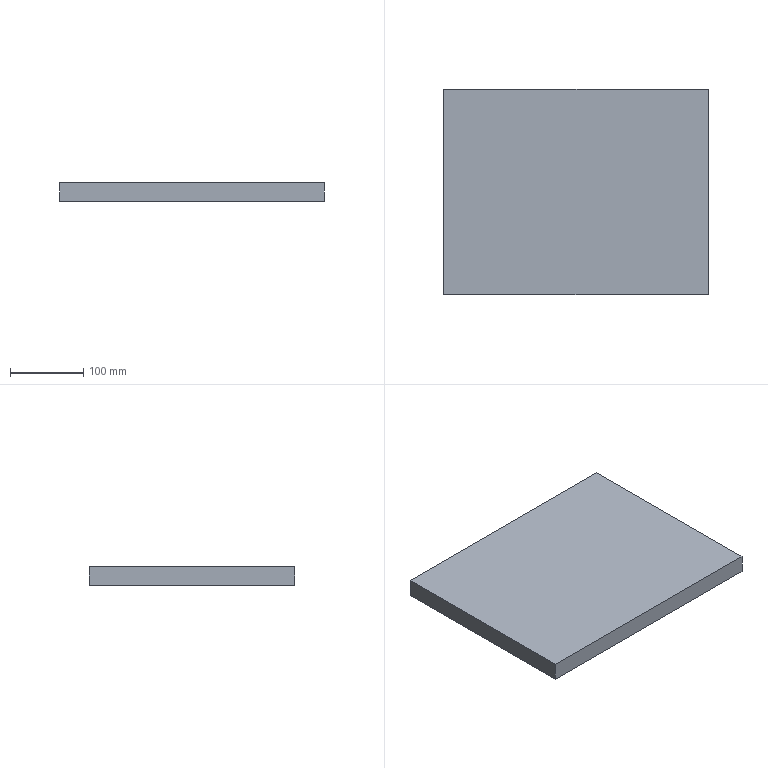Part | SolidWorks | features Extrusion 1 | 1 solid | 6 faces | box 360 x 280 x 25 mm | volume 2520000 mm3 | plane 6
STEP:
#1=CARTESIAN_POINT('',(180.,-140.,0.));
#2=VERTEX_POINT('',#1);
#3=CARTESIAN_POINT('',(180.,140.,0.));
#4=VERTEX_POINT('',#3);
#5=CARTESIAN_POINT('',(180.,140.,0.));
#6=DIRECTION('',(0.,1.,0.));
#7=VECTOR('',#6,1000.);
#8=LINE('',#5,#7);
#9=EDGE_CURVE('',#2,#4,#8,.T.);
#10=ORIENTED_EDGE('',*,*,#9,.T.);
#11=CARTESIAN_POINT('',(180.,140.,25.));
#12=VERTEX_POINT('',#11);
#13=CARTESIAN_POINT('',(180.,140.,25.));
#14=DIRECTION('',(0.,0.,-1.));
#15=VECTOR('',#14,1000.);
#16=LINE('',#13,#15);
#17=EDGE_CURVE('',#12,#4,#16,.T.);
#18=ORIENTED_EDGE('',*,*,#17,.F.);
#19=CARTESIAN_POINT('',(180.,-140.,25.));
#20=VERTEX_POINT('',#19);
#21=CARTESIAN_POINT('',(180.,140.,25.));
#22=DIRECTION('',(0.,1.,0.));
#23=VECTOR('',#22,1000.);
#24=LINE('',#21,#23);
#25=EDGE_CURVE('',#20,#12,#24,.T.);
#26=ORIENTED_EDGE('',*,*,#25,.F.);
#27=CARTESIAN_POINT('',(180.,-140.,25.));
#28=DIRECTION('',(0.,0.,-1.));
#29=VECTOR('',#28,1000.);
#30=LINE('',#27,#29);
#31=EDGE_CURVE('',#20,#2,#30,.T.);
#32=ORIENTED_EDGE('',*,*,#31,.T.);
#33=EDGE_LOOP('',(#10,#18,#26,#32));
#34=FACE_OUTER_BOUND('',#33,.T.);
#35=CARTESIAN_POINT('',(180.,140.,25.));
#36=DIRECTION('',(-1.,0.,0.));
#37=DIRECTION('',(0.,-1.,0.));
#38=AXIS2_PLACEMENT_3D('',#35,#36,#37);
#39=PLANE('',#38);
#40=ADVANCED_FACE('',(#34),#39,.F.);
#41=CARTESIAN_POINT('',(-180.,140.,0.));
#42=VERTEX_POINT('',#41);
#43=CARTESIAN_POINT('',(-180.,140.,0.));
#44=DIRECTION('',(-1.,0.,0.));
#45=VECTOR('',#44,1000.);
#46=LINE('',#43,#45);
#47=EDGE_CURVE('',#4,#42,#46,.T.);
#48=ORIENTED_EDGE('',*,*,#47,.T.);
#49=CARTESIAN_POINT('',(-180.,140.,25.));
#50=VERTEX_POINT('',#49);
#51=CARTESIAN_POINT('',(-180.,140.,25.));
#52=DIRECTION('',(0.,0.,-1.));
#53=VECTOR('',#52,1000.);
#54=LINE('',#51,#53);
#55=EDGE_CURVE('',#50,#42,#54,.T.);
#56=ORIENTED_EDGE('',*,*,#55,.F.);
#57=CARTESIAN_POINT('',(-180.,140.,25.));
#58=DIRECTION('',(-1.,0.,0.));
#59=VECTOR('',#58,1000.);
#60=LINE('',#57,#59);
#61=EDGE_CURVE('',#12,#50,#60,.T.);
#62=ORIENTED_EDGE('',*,*,#61,.F.);
#63=ORIENTED_EDGE('',*,*,#17,.T.);
#64=EDGE_LOOP('',(#48,#56,#62,#63));
#65=FACE_OUTER_BOUND('',#64,.T.);
#66=CARTESIAN_POINT('',(-180.,140.,25.));
#67=DIRECTION('',(0.,-1.,0.));
#68=DIRECTION('',(0.,0.,-1.));
#69=AXIS2_PLACEMENT_3D('',#66,#67,#68);
#70=PLANE('',#69);
#71=ADVANCED_FACE('',(#65),#70,.F.);
#72=CARTESIAN_POINT('',(-180.,-140.,0.));
#73=VERTEX_POINT('',#72);
#74=CARTESIAN_POINT('',(-180.,140.,0.));
#75=DIRECTION('',(0.,-1.,0.));
#76=VECTOR('',#75,1000.);
#77=LINE('',#74,#76);
#78=EDGE_CURVE('',#42,#73,#77,.T.);
#79=ORIENTED_EDGE('',*,*,#78,.T.);
#80=CARTESIAN_POINT('',(-180.,-140.,25.));
#81=VERTEX_POINT('',#80);
#82=CARTESIAN_POINT('',(-180.,-140.,25.));
#83=DIRECTION('',(0.,0.,-1.));
#84=VECTOR('',#83,1000.);
#85=LINE('',#82,#84);
#86=EDGE_CURVE('',#81,#73,#85,.T.);
#87=ORIENTED_EDGE('',*,*,#86,.F.);
#88=CARTESIAN_POINT('',(-180.,140.,25.));
#89=DIRECTION('',(0.,-1.,0.));
#90=VECTOR('',#89,1000.);
#91=LINE('',#88,#90);
#92=EDGE_CURVE('',#50,#81,#91,.T.);
#93=ORIENTED_EDGE('',*,*,#92,.F.);
#94=ORIENTED_EDGE('',*,*,#55,.T.);
#95=EDGE_LOOP('',(#79,#87,#93,#94));
#96=FACE_OUTER_BOUND('',#95,.T.);
#97=CARTESIAN_POINT('',(-180.,140.,25.));
#98=DIRECTION('',(1.,0.,0.));
#99=DIRECTION('',(0.,1.,0.));
#100=AXIS2_PLACEMENT_3D('',#97,#98,#99);
#101=PLANE('',#100);
#102=ADVANCED_FACE('',(#96),#101,.F.);
#103=CARTESIAN_POINT('',(-180.,-140.,0.));
#104=DIRECTION('',(1.,0.,0.));
#105=VECTOR('',#104,1000.);
#106=LINE('',#103,#105);
#107=EDGE_CURVE('',#73,#2,#106,.T.);
#108=ORIENTED_EDGE('',*,*,#107,.T.);
#109=ORIENTED_EDGE('',*,*,#31,.F.);
#110=CARTESIAN_POINT('',(-180.,-140.,25.));
#111=DIRECTION('',(1.,0.,0.));
#112=VECTOR('',#111,1000.);
#113=LINE('',#110,#112);
#114=EDGE_CURVE('',#81,#20,#113,.T.);
#115=ORIENTED_EDGE('',*,*,#114,.F.);
#116=ORIENTED_EDGE('',*,*,#86,.T.);
#117=EDGE_LOOP('',(#108,#109,#115,#116));
#118=FACE_OUTER_BOUND('',#117,.T.);
#119=CARTESIAN_POINT('',(-180.,-140.,25.));
#120=DIRECTION('',(0.,1.,0.));
#121=DIRECTION('',(0.,0.,1.));
#122=AXIS2_PLACEMENT_3D('',#119,#120,#121);
#123=PLANE('',#122);
#124=ADVANCED_FACE('',(#118),#123,.F.);
#125=ORIENTED_EDGE('',*,*,#25,.T.);
#126=ORIENTED_EDGE('',*,*,#61,.T.);
#127=ORIENTED_EDGE('',*,*,#92,.T.);
#128=ORIENTED_EDGE('',*,*,#114,.T.);
#129=EDGE_LOOP('',(#125,#126,#127,#128));
#130=FACE_OUTER_BOUND('',#129,.T.);
#131=CARTESIAN_POINT('',(0.,0.,25.));
#132=DIRECTION('',(0.,0.,1.));
#133=DIRECTION('',(1.,0.,0.));
#134=AXIS2_PLACEMENT_3D('',#131,#132,#133);
#135=PLANE('',#134);
#136=ADVANCED_FACE('',(#130),#135,.T.);
#137=ORIENTED_EDGE('',*,*,#9,.F.);
#138=ORIENTED_EDGE('',*,*,#107,.F.);
#139=ORIENTED_EDGE('',*,*,#78,.F.);
#140=ORIENTED_EDGE('',*,*,#47,.F.);
#141=EDGE_LOOP('',(#137,#138,#139,#140));
#142=FACE_OUTER_BOUND('',#141,.T.);
#143=CARTESIAN_POINT('',(0.,0.,0.));
#144=DIRECTION('',(0.,0.,1.));
#145=DIRECTION('',(1.,0.,0.));
#146=AXIS2_PLACEMENT_3D('',#143,#144,#145);
#147=PLANE('',#146);
#148=ADVANCED_FACE('',(#142),#147,.F.);
#149=CLOSED_SHELL('',(#40,#71,#102,#124,#136,#148));
#150=MANIFOLD_SOLID_BREP('',#149);
#151=CARTESIAN_POINT('',(0.,0.,0.));
#152=DIRECTION('',(0.,0.,1.));
#153=DIRECTION('',(1.,0.,0.));
#154=AXIS2_PLACEMENT_3D('',#151,#152,#153);
#155=(LENGTH_UNIT()NAMED_UNIT(*)SI_UNIT(.MILLI.,.METRE.));
#156=UNCERTAINTY_MEASURE_WITH_UNIT(LENGTH_MEASURE(0.00001),#155,'','');
#157=(NAMED_UNIT(*)PLANE_ANGLE_UNIT()SI_UNIT($,.RADIAN.));
#158=(NAMED_UNIT(*)SI_UNIT($,.STERADIAN.)SOLID_ANGLE_UNIT());
#159=(GEOMETRIC_REPRESENTATION_CONTEXT(3)GLOBAL_UNCERTAINTY_ASSIGNED_CONTEXT((#156))GLOBAL_UNIT_ASSIGNED_CONTEXT((#155,#157,#158))REPRESENTATION_CONTEXT('',''));
#160=ADVANCED_BREP_SHAPE_REPRESENTATION('',(#150,#154),#159);